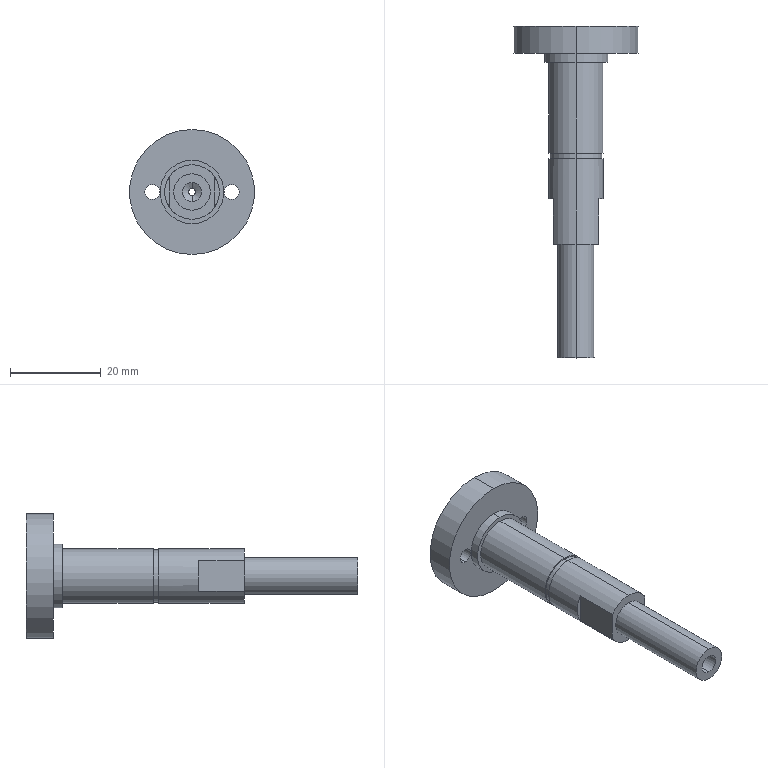Part | STEP file | PN_0037 | 1 solid | 39 faces | box 27.5 x 73 x 27.5 mm | volume 9090 mm3 | cylinder 24 | plane 13 | cone 2 | commonest cylinder face diameters 12 x6 3.3 x4 8 x4 1.5 x2 4.2 x2 11.5 x2